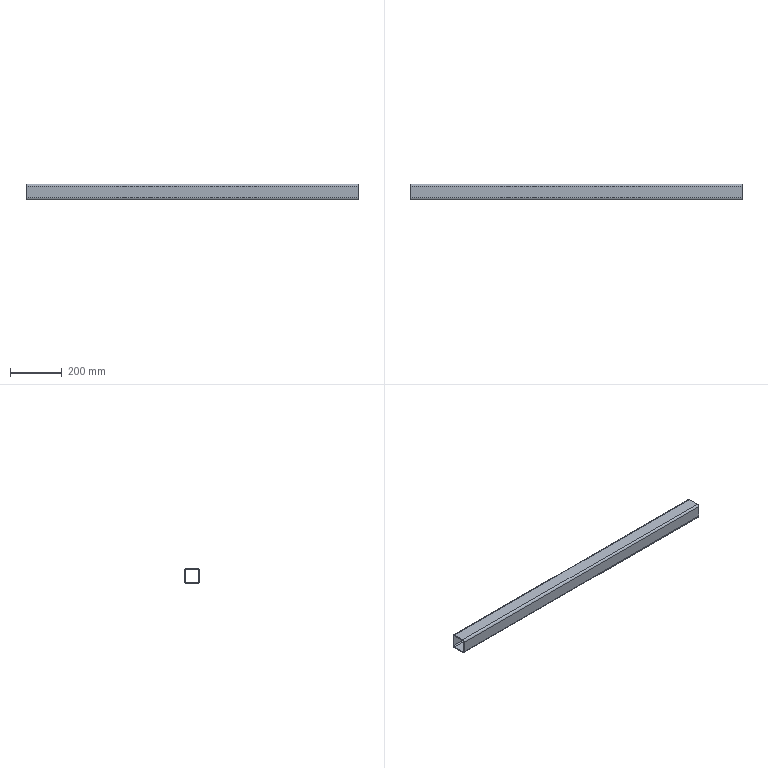Part | SolidWorks | features BaseBody 1 | 1 solid | 18 faces | box 1280 x 60 x 60 mm | volume 1094139 mm3 | plane 10 | cylinder 8 | commonest cylinder face diameters 8 x4 16 x4
STEP:
#1=CARTESIAN_POINT('',(640.,44.,-4.));
#2=VERTEX_POINT('',#1);
#3=CARTESIAN_POINT('',(640.,0.,-4.));
#4=VERTEX_POINT('',#3);
#5=CARTESIAN_POINT('',(640.,44.,-4.));
#6=DIRECTION('',(0.,-1.,0.));
#7=VECTOR('',#6,1000.);
#8=LINE('',#5,#7);
#9=EDGE_CURVE('',#2,#4,#8,.T.);
#10=ORIENTED_EDGE('',*,*,#9,.T.);
#11=CARTESIAN_POINT('',(-640.,0.,-4.));
#12=VERTEX_POINT('',#11);
#13=CARTESIAN_POINT('',(670.,0.,-4.));
#14=DIRECTION('',(-1.,0.,0.));
#15=VECTOR('',#14,1000.);
#16=LINE('',#13,#15);
#17=EDGE_CURVE('',#4,#12,#16,.T.);
#18=ORIENTED_EDGE('',*,*,#17,.T.);
#19=CARTESIAN_POINT('',(-640.,44.,-4.));
#20=VERTEX_POINT('',#19);
#21=CARTESIAN_POINT('',(-640.,44.,-4.));
#22=DIRECTION('',(0.,1.,0.));
#23=VECTOR('',#22,1000.);
#24=LINE('',#21,#23);
#25=EDGE_CURVE('',#12,#20,#24,.T.);
#26=ORIENTED_EDGE('',*,*,#25,.T.);
#27=CARTESIAN_POINT('',(670.,44.,-4.));
#28=DIRECTION('',(1.,0.,0.));
#29=VECTOR('',#28,1000.);
#30=LINE('',#27,#29);
#31=EDGE_CURVE('',#20,#2,#30,.T.);
#32=ORIENTED_EDGE('',*,*,#31,.T.);
#33=EDGE_LOOP('',(#10,#18,#26,#32));
#34=FACE_OUTER_BOUND('',#33,.T.);
#35=CARTESIAN_POINT('',(670.,44.,-4.));
#36=DIRECTION('',(0.,0.,-1.));
#37=DIRECTION('',(-1.,0.,0.));
#38=AXIS2_PLACEMENT_3D('',#35,#36,#37);
#39=PLANE('',#38);
#40=ADVANCED_FACE('',(#34),#39,.T.);
#41=ORIENTED_EDGE('',*,*,#17,.F.);
#42=CARTESIAN_POINT('',(640.,-4.,-8.));
#43=VERTEX_POINT('',#42);
#44=CARTESIAN_POINT('',(640.,0.,-8.));
#45=DIRECTION('',(-1.,0.,0.));
#46=DIRECTION('',(0.,0.,1.));
#47=AXIS2_PLACEMENT_3D('',#44,#45,#46);
#48=CIRCLE('',#47,4.);
#49=EDGE_CURVE('',#43,#4,#48,.T.);
#50=ORIENTED_EDGE('',*,*,#49,.F.);
#51=CARTESIAN_POINT('',(-640.,-4.,-8.));
#52=VERTEX_POINT('',#51);
#53=CARTESIAN_POINT('',(670.,-4.,-8.));
#54=DIRECTION('',(1.,0.,0.));
#55=VECTOR('',#54,1000.);
#56=LINE('',#53,#55);
#57=EDGE_CURVE('',#52,#43,#56,.T.);
#58=ORIENTED_EDGE('',*,*,#57,.F.);
#59=CARTESIAN_POINT('',(-640.,0.,-8.));
#60=DIRECTION('',(1.,0.,0.));
#61=DIRECTION('',(0.,0.,1.));
#62=AXIS2_PLACEMENT_3D('',#59,#60,#61);
#63=CIRCLE('',#62,4.);
#64=EDGE_CURVE('',#12,#52,#63,.T.);
#65=ORIENTED_EDGE('',*,*,#64,.F.);
#66=EDGE_LOOP('',(#41,#50,#58,#65));
#67=FACE_OUTER_BOUND('',#66,.T.);
#68=CARTESIAN_POINT('',(670.,0.,-8.));
#69=DIRECTION('',(-1.,0.,0.));
#70=DIRECTION('',(0.,0.,1.));
#71=AXIS2_PLACEMENT_3D('',#68,#69,#70);
#72=CYLINDRICAL_SURFACE('',#71,4.);
#73=ADVANCED_FACE('',(#67),#72,.F.);
#74=ORIENTED_EDGE('',*,*,#49,.T.);
#75=ORIENTED_EDGE('',*,*,#9,.F.);
#76=CARTESIAN_POINT('',(640.,48.,-8.));
#77=VERTEX_POINT('',#76);
#78=CARTESIAN_POINT('',(640.,44.,-8.));
#79=DIRECTION('',(-1.,0.,0.));
#80=DIRECTION('',(0.,0.,1.));
#81=AXIS2_PLACEMENT_3D('',#78,#79,#80);
#82=CIRCLE('',#81,4.);
#83=EDGE_CURVE('',#2,#77,#82,.T.);
#84=ORIENTED_EDGE('',*,*,#83,.T.);
#85=CARTESIAN_POINT('',(640.,48.,-52.));
#86=VERTEX_POINT('',#85);
#87=CARTESIAN_POINT('',(640.,48.,530.));
#88=DIRECTION('',(0.,0.,-1.));
#89=VECTOR('',#88,1000.);
#90=LINE('',#87,#89);
#91=EDGE_CURVE('',#77,#86,#90,.T.);
#92=ORIENTED_EDGE('',*,*,#91,.T.);
#93=CARTESIAN_POINT('',(640.,44.,-56.));
#94=VERTEX_POINT('',#93);
#95=CARTESIAN_POINT('',(640.,44.,-52.));
#96=DIRECTION('',(-1.,0.,0.));
#97=DIRECTION('',(0.,0.,1.));
#98=AXIS2_PLACEMENT_3D('',#95,#96,#97);
#99=CIRCLE('',#98,4.);
#100=EDGE_CURVE('',#86,#94,#99,.T.);
#101=ORIENTED_EDGE('',*,*,#100,.T.);
#102=CARTESIAN_POINT('',(640.,0.,-56.));
#103=VERTEX_POINT('',#102);
#104=CARTESIAN_POINT('',(640.,44.,-56.));
#105=DIRECTION('',(0.,-1.,0.));
#106=VECTOR('',#105,1000.);
#107=LINE('',#104,#106);
#108=EDGE_CURVE('',#94,#103,#107,.T.);
#109=ORIENTED_EDGE('',*,*,#108,.T.);
#110=CARTESIAN_POINT('',(640.,-4.,-52.));
#111=VERTEX_POINT('',#110);
#112=CARTESIAN_POINT('',(640.,0.,-52.));
#113=DIRECTION('',(-1.,0.,0.));
#114=DIRECTION('',(0.,0.,1.));
#115=AXIS2_PLACEMENT_3D('',#112,#113,#114);
#116=CIRCLE('',#115,4.);
#117=EDGE_CURVE('',#103,#111,#116,.T.);
#118=ORIENTED_EDGE('',*,*,#117,.T.);
#119=CARTESIAN_POINT('',(640.,-4.,530.));
#120=DIRECTION('',(0.,0.,1.));
#121=VECTOR('',#120,1000.);
#122=LINE('',#119,#121);
#123=EDGE_CURVE('',#111,#43,#122,.T.);
#124=ORIENTED_EDGE('',*,*,#123,.T.);
#125=EDGE_LOOP('',(#74,#75,#84,#92,#101,#109,#118,#124));
#126=FACE_BOUND('',#125,.T.);
#127=CARTESIAN_POINT('',(640.,52.,-52.));
#128=VERTEX_POINT('',#127);
#129=CARTESIAN_POINT('',(640.,52.,-8.));
#130=VERTEX_POINT('',#129);
#131=CARTESIAN_POINT('',(640.,52.,530.));
#132=DIRECTION('',(0.,0.,1.));
#133=VECTOR('',#132,1000.);
#134=LINE('',#131,#133);
#135=EDGE_CURVE('',#128,#130,#134,.T.);
#136=ORIENTED_EDGE('',*,*,#135,.T.);
#137=CARTESIAN_POINT('',(640.,44.,0.));
#138=VERTEX_POINT('',#137);
#139=CARTESIAN_POINT('',(640.,44.,-8.));
#140=DIRECTION('',(1.,0.,0.));
#141=DIRECTION('',(0.,0.,1.));
#142=AXIS2_PLACEMENT_3D('',#139,#140,#141);
#143=CIRCLE('',#142,8.);
#144=EDGE_CURVE('',#130,#138,#143,.T.);
#145=ORIENTED_EDGE('',*,*,#144,.T.);
#146=CARTESIAN_POINT('',(640.,0.,0.));
#147=VERTEX_POINT('',#146);
#148=CARTESIAN_POINT('',(640.,44.,0.));
#149=DIRECTION('',(0.,-1.,0.));
#150=VECTOR('',#149,1000.);
#151=LINE('',#148,#150);
#152=EDGE_CURVE('',#138,#147,#151,.T.);
#153=ORIENTED_EDGE('',*,*,#152,.T.);
#154=CARTESIAN_POINT('',(640.,-8.,-8.));
#155=VERTEX_POINT('',#154);
#156=CARTESIAN_POINT('',(640.,0.,-8.));
#157=DIRECTION('',(1.,0.,0.));
#158=DIRECTION('',(0.,0.,1.));
#159=AXIS2_PLACEMENT_3D('',#156,#157,#158);
#160=CIRCLE('',#159,8.);
#161=EDGE_CURVE('',#147,#155,#160,.T.);
#162=ORIENTED_EDGE('',*,*,#161,.T.);
#163=CARTESIAN_POINT('',(640.,-8.,-52.));
#164=VERTEX_POINT('',#163);
#165=CARTESIAN_POINT('',(640.,-8.,530.));
#166=DIRECTION('',(0.,0.,-1.));
#167=VECTOR('',#166,1000.);
#168=LINE('',#165,#167);
#169=EDGE_CURVE('',#155,#164,#168,.T.);
#170=ORIENTED_EDGE('',*,*,#169,.T.);
#171=CARTESIAN_POINT('',(640.,0.,-60.));
#172=VERTEX_POINT('',#171);
#173=CARTESIAN_POINT('',(640.,0.,-52.));
#174=DIRECTION('',(1.,0.,0.));
#175=DIRECTION('',(0.,0.,1.));
#176=AXIS2_PLACEMENT_3D('',#173,#174,#175);
#177=CIRCLE('',#176,8.);
#178=EDGE_CURVE('',#164,#172,#177,.T.);
#179=ORIENTED_EDGE('',*,*,#178,.T.);
#180=CARTESIAN_POINT('',(640.,44.,-60.));
#181=VERTEX_POINT('',#180);
#182=CARTESIAN_POINT('',(640.,44.,-60.));
#183=DIRECTION('',(0.,1.,0.));
#184=VECTOR('',#183,1000.);
#185=LINE('',#182,#184);
#186=EDGE_CURVE('',#172,#181,#185,.T.);
#187=ORIENTED_EDGE('',*,*,#186,.T.);
#188=CARTESIAN_POINT('',(640.,44.,-52.));
#189=DIRECTION('',(1.,0.,0.));
#190=DIRECTION('',(0.,0.,1.));
#191=AXIS2_PLACEMENT_3D('',#188,#189,#190);
#192=CIRCLE('',#191,8.);
#193=EDGE_CURVE('',#181,#128,#192,.T.);
#194=ORIENTED_EDGE('',*,*,#193,.T.);
#195=EDGE_LOOP('',(#136,#145,#153,#162,#170,#179,#187,#194));
#196=FACE_OUTER_BOUND('',#195,.T.);
#197=CARTESIAN_POINT('',(640.,44.,530.));
#198=DIRECTION('',(1.,0.,0.));
#199=DIRECTION('',(0.,0.,-1.));
#200=AXIS2_PLACEMENT_3D('',#197,#198,#199);
#201=PLANE('',#200);
#202=ADVANCED_FACE('',(#126,#196),#201,.T.);
#203=CARTESIAN_POINT('',(-640.,48.,-8.));
#204=VERTEX_POINT('',#203);
#205=CARTESIAN_POINT('',(670.,48.,-8.));
#206=DIRECTION('',(-1.,0.,0.));
#207=VECTOR('',#206,1000.);
#208=LINE('',#205,#207);
#209=EDGE_CURVE('',#77,#204,#208,.T.);
#210=ORIENTED_EDGE('',*,*,#209,.F.);
#211=ORIENTED_EDGE('',*,*,#83,.F.);
#212=ORIENTED_EDGE('',*,*,#31,.F.);
#213=CARTESIAN_POINT('',(-640.,44.,-8.));
#214=DIRECTION('',(1.,0.,0.));
#215=DIRECTION('',(0.,0.,1.));
#216=AXIS2_PLACEMENT_3D('',#213,#214,#215);
#217=CIRCLE('',#216,4.);
#218=EDGE_CURVE('',#204,#20,#217,.T.);
#219=ORIENTED_EDGE('',*,*,#218,.F.);
#220=EDGE_LOOP('',(#210,#211,#212,#219));
#221=FACE_OUTER_BOUND('',#220,.T.);
#222=CARTESIAN_POINT('',(670.,44.,-8.));
#223=DIRECTION('',(-1.,0.,0.));
#224=DIRECTION('',(0.,0.,1.));
#225=AXIS2_PLACEMENT_3D('',#222,#223,#224);
#226=CYLINDRICAL_SURFACE('',#225,4.);
#227=ADVANCED_FACE('',(#221),#226,.F.);
#228=CARTESIAN_POINT('',(-640.,-4.,-52.));
#229=VERTEX_POINT('',#228);
#230=CARTESIAN_POINT('',(-640.,-4.,530.));
#231=DIRECTION('',(0.,0.,-1.));
#232=VECTOR('',#231,1000.);
#233=LINE('',#230,#232);
#234=EDGE_CURVE('',#52,#229,#233,.T.);
#235=ORIENTED_EDGE('',*,*,#234,.T.);
#236=CARTESIAN_POINT('',(-640.,0.,-56.));
#237=VERTEX_POINT('',#236);
#238=CARTESIAN_POINT('',(-640.,0.,-52.));
#239=DIRECTION('',(1.,0.,0.));
#240=DIRECTION('',(0.,0.,1.));
#241=AXIS2_PLACEMENT_3D('',#238,#239,#240);
#242=CIRCLE('',#241,4.);
#243=EDGE_CURVE('',#229,#237,#242,.T.);
#244=ORIENTED_EDGE('',*,*,#243,.T.);
#245=CARTESIAN_POINT('',(-640.,44.,-56.));
#246=VERTEX_POINT('',#245);
#247=CARTESIAN_POINT('',(-640.,0.,-56.));
#248=DIRECTION('',(0.,1.,0.));
#249=VECTOR('',#248,1000.);
#250=LINE('',#247,#249);
#251=EDGE_CURVE('',#237,#246,#250,.T.);
#252=ORIENTED_EDGE('',*,*,#251,.T.);
#253=CARTESIAN_POINT('',(-640.,48.,-52.));
#254=VERTEX_POINT('',#253);
#255=CARTESIAN_POINT('',(-640.,44.,-52.));
#256=DIRECTION('',(1.,0.,0.));
#257=DIRECTION('',(0.,0.,1.));
#258=AXIS2_PLACEMENT_3D('',#255,#256,#257);
#259=CIRCLE('',#258,4.);
#260=EDGE_CURVE('',#246,#254,#259,.T.);
#261=ORIENTED_EDGE('',*,*,#260,.T.);
#262=CARTESIAN_POINT('',(-640.,48.,530.));
#263=DIRECTION('',(0.,0.,1.));
#264=VECTOR('',#263,1000.);
#265=LINE('',#262,#264);
#266=EDGE_CURVE('',#254,#204,#265,.T.);
#267=ORIENTED_EDGE('',*,*,#266,.T.);
#268=ORIENTED_EDGE('',*,*,#218,.T.);
#269=ORIENTED_EDGE('',*,*,#25,.F.);
#270=ORIENTED_EDGE('',*,*,#64,.T.);
#271=EDGE_LOOP('',(#235,#244,#252,#261,#267,#268,#269,#270));
#272=FACE_BOUND('',#271,.T.);
#273=CARTESIAN_POINT('',(-640.,52.,-8.));
#274=VERTEX_POINT('',#273);
#275=CARTESIAN_POINT('',(-640.,52.,-52.));
#276=VERTEX_POINT('',#275);
#277=CARTESIAN_POINT('',(-640.,52.,530.));
#278=DIRECTION('',(0.,0.,-1.));
#279=VECTOR('',#278,1000.);
#280=LINE('',#277,#279);
#281=EDGE_CURVE('',#274,#276,#280,.T.);
#282=ORIENTED_EDGE('',*,*,#281,.T.);
#283=CARTESIAN_POINT('',(-640.,44.,-60.));
#284=VERTEX_POINT('',#283);
#285=CARTESIAN_POINT('',(-640.,44.,-52.));
#286=DIRECTION('',(-1.,0.,0.));
#287=DIRECTION('',(0.,0.,1.));
#288=AXIS2_PLACEMENT_3D('',#285,#286,#287);
#289=CIRCLE('',#288,8.);
#290=EDGE_CURVE('',#276,#284,#289,.T.);
#291=ORIENTED_EDGE('',*,*,#290,.T.);
#292=CARTESIAN_POINT('',(-640.,0.,-60.));
#293=VERTEX_POINT('',#292);
#294=CARTESIAN_POINT('',(-640.,0.,-60.));
#295=DIRECTION('',(0.,-1.,0.));
#296=VECTOR('',#295,1000.);
#297=LINE('',#294,#296);
#298=EDGE_CURVE('',#284,#293,#297,.T.);
#299=ORIENTED_EDGE('',*,*,#298,.T.);
#300=CARTESIAN_POINT('',(-640.,-8.,-52.));
#301=VERTEX_POINT('',#300);
#302=CARTESIAN_POINT('',(-640.,0.,-52.));
#303=DIRECTION('',(-1.,0.,0.));
#304=DIRECTION('',(0.,0.,1.));
#305=AXIS2_PLACEMENT_3D('',#302,#303,#304);
#306=CIRCLE('',#305,8.);
#307=EDGE_CURVE('',#293,#301,#306,.T.);
#308=ORIENTED_EDGE('',*,*,#307,.T.);
#309=CARTESIAN_POINT('',(-640.,-8.,-8.));
#310=VERTEX_POINT('',#309);
#311=CARTESIAN_POINT('',(-640.,-8.,530.));
#312=DIRECTION('',(0.,0.,1.));
#313=VECTOR('',#312,1000.);
#314=LINE('',#311,#313);
#315=EDGE_CURVE('',#301,#310,#314,.T.);
#316=ORIENTED_EDGE('',*,*,#315,.T.);
#317=CARTESIAN_POINT('',(-640.,0.,0.));
#318=VERTEX_POINT('',#317);
#319=CARTESIAN_POINT('',(-640.,0.,-8.));
#320=DIRECTION('',(-1.,0.,0.));
#321=DIRECTION('',(0.,0.,1.));
#322=AXIS2_PLACEMENT_3D('',#319,#320,#321);
#323=CIRCLE('',#322,8.);
#324=EDGE_CURVE('',#310,#318,#323,.T.);
#325=ORIENTED_EDGE('',*,*,#324,.T.);
#326=CARTESIAN_POINT('',(-640.,44.,0.));
#327=VERTEX_POINT('',#326);
#328=CARTESIAN_POINT('',(-640.,0.,0.));
#329=DIRECTION('',(0.,1.,0.));
#330=VECTOR('',#329,1000.);
#331=LINE('',#328,#330);
#332=EDGE_CURVE('',#318,#327,#331,.T.);
#333=ORIENTED_EDGE('',*,*,#332,.T.);
#334=CARTESIAN_POINT('',(-640.,44.,-8.));
#335=DIRECTION('',(-1.,0.,0.));
#336=DIRECTION('',(0.,0.,1.));
#337=AXIS2_PLACEMENT_3D('',#334,#335,#336);
#338=CIRCLE('',#337,8.);
#339=EDGE_CURVE('',#327,#274,#338,.T.);
#340=ORIENTED_EDGE('',*,*,#339,.T.);
#341=EDGE_LOOP('',(#282,#291,#299,#308,#316,#325,#333,#340));
#342=FACE_OUTER_BOUND('',#341,.T.);
#343=CARTESIAN_POINT('',(-640.,0.,530.));
#344=DIRECTION('',(-1.,0.,0.));
#345=DIRECTION('',(0.,0.,1.));
#346=AXIS2_PLACEMENT_3D('',#343,#344,#345);
#347=PLANE('',#346);
#348=ADVANCED_FACE('',(#272,#342),#347,.T.);
#349=ORIENTED_EDGE('',*,*,#123,.F.);
#350=CARTESIAN_POINT('',(670.,-4.,-52.));
#351=DIRECTION('',(-1.,0.,0.));
#352=VECTOR('',#351,1000.);
#353=LINE('',#350,#352);
#354=EDGE_CURVE('',#111,#229,#353,.T.);
#355=ORIENTED_EDGE('',*,*,#354,.T.);
#356=ORIENTED_EDGE('',*,*,#234,.F.);
#357=ORIENTED_EDGE('',*,*,#57,.T.);
#358=EDGE_LOOP('',(#349,#355,#356,#357));
#359=FACE_OUTER_BOUND('',#358,.T.);
#360=CARTESIAN_POINT('',(670.,-4.,-52.));
#361=DIRECTION('',(0.,1.,0.));
#362=DIRECTION('',(0.,0.,1.));
#363=AXIS2_PLACEMENT_3D('',#360,#361,#362);
#364=PLANE('',#363);
#365=ADVANCED_FACE('',(#359),#364,.T.);
#366=ORIENTED_EDGE('',*,*,#354,.F.);
#367=ORIENTED_EDGE('',*,*,#117,.F.);
#368=CARTESIAN_POINT('',(670.,0.,-56.));
#369=DIRECTION('',(1.,0.,0.));
#370=VECTOR('',#369,1000.);
#371=LINE('',#368,#370);
#372=EDGE_CURVE('',#237,#103,#371,.T.);
#373=ORIENTED_EDGE('',*,*,#372,.F.);
#374=ORIENTED_EDGE('',*,*,#243,.F.);
#375=EDGE_LOOP('',(#366,#367,#373,#374));
#376=FACE_OUTER_BOUND('',#375,.T.);
#377=CARTESIAN_POINT('',(670.,0.,-52.));
#378=DIRECTION('',(-1.,0.,0.));
#379=DIRECTION('',(0.,0.,1.));
#380=AXIS2_PLACEMENT_3D('',#377,#378,#379);
#381=CYLINDRICAL_SURFACE('',#380,4.);
#382=ADVANCED_FACE('',(#376),#381,.F.);
#383=ORIENTED_EDGE('',*,*,#108,.F.);
#384=CARTESIAN_POINT('',(670.,44.,-56.));
#385=DIRECTION('',(-1.,0.,0.));
#386=VECTOR('',#385,1000.);
#387=LINE('',#384,#386);
#388=EDGE_CURVE('',#94,#246,#387,.T.);
#389=ORIENTED_EDGE('',*,*,#388,.T.);
#390=ORIENTED_EDGE('',*,*,#251,.F.);
#391=ORIENTED_EDGE('',*,*,#372,.T.);
#392=EDGE_LOOP('',(#383,#389,#390,#391));
#393=FACE_OUTER_BOUND('',#392,.T.);
#394=CARTESIAN_POINT('',(670.,0.,-56.));
#395=DIRECTION('',(0.,0.,1.));
#396=DIRECTION('',(1.,0.,0.));
#397=AXIS2_PLACEMENT_3D('',#394,#395,#396);
#398=PLANE('',#397);
#399=ADVANCED_FACE('',(#393),#398,.T.);
#400=ORIENTED_EDGE('',*,*,#388,.F.);
#401=ORIENTED_EDGE('',*,*,#100,.F.);
#402=CARTESIAN_POINT('',(670.,48.,-52.));
#403=DIRECTION('',(1.,0.,0.));
#404=VECTOR('',#403,1000.);
#405=LINE('',#402,#404);
#406=EDGE_CURVE('',#254,#86,#405,.T.);
#407=ORIENTED_EDGE('',*,*,#406,.F.);
#408=ORIENTED_EDGE('',*,*,#260,.F.);
#409=EDGE_LOOP('',(#400,#401,#407,#408));
#410=FACE_OUTER_BOUND('',#409,.T.);
#411=CARTESIAN_POINT('',(670.,44.,-52.));
#412=DIRECTION('',(-1.,0.,0.));
#413=DIRECTION('',(0.,0.,1.));
#414=AXIS2_PLACEMENT_3D('',#411,#412,#413);
#415=CYLINDRICAL_SURFACE('',#414,4.);
#416=ADVANCED_FACE('',(#410),#415,.F.);
#417=ORIENTED_EDGE('',*,*,#91,.F.);
#418=ORIENTED_EDGE('',*,*,#209,.T.);
#419=ORIENTED_EDGE('',*,*,#266,.F.);
#420=ORIENTED_EDGE('',*,*,#406,.T.);
#421=EDGE_LOOP('',(#417,#418,#419,#420));
#422=FACE_OUTER_BOUND('',#421,.T.);
#423=CARTESIAN_POINT('',(670.,48.,-8.));
#424=DIRECTION('',(0.,-1.,0.));
#425=DIRECTION('',(0.,0.,-1.));
#426=AXIS2_PLACEMENT_3D('',#423,#424,#425);
#427=PLANE('',#426);
#428=ADVANCED_FACE('',(#422),#427,.T.);
#429=CARTESIAN_POINT('',(670.,52.,-8.));
#430=DIRECTION('',(-1.,0.,0.));
#431=VECTOR('',#430,1000.);
#432=LINE('',#429,#431);
#433=EDGE_CURVE('',#130,#274,#432,.T.);
#434=ORIENTED_EDGE('',*,*,#433,.T.);
#435=ORIENTED_EDGE('',*,*,#339,.F.);
#436=CARTESIAN_POINT('',(670.,44.,0.));
#437=DIRECTION('',(1.,0.,0.));
#438=VECTOR('',#437,1000.);
#439=LINE('',#436,#438);
#440=EDGE_CURVE('',#327,#138,#439,.T.);
#441=ORIENTED_EDGE('',*,*,#440,.T.);
#442=ORIENTED_EDGE('',*,*,#144,.F.);
#443=EDGE_LOOP('',(#434,#435,#441,#442));
#444=FACE_OUTER_BOUND('',#443,.T.);
#445=CARTESIAN_POINT('',(670.,44.,-8.));
#446=DIRECTION('',(-1.,0.,0.));
#447=DIRECTION('',(0.,0.,1.));
#448=AXIS2_PLACEMENT_3D('',#445,#446,#447);
#449=CYLINDRICAL_SURFACE('',#448,8.);
#450=ADVANCED_FACE('',(#444),#449,.T.);
#451=ORIENTED_EDGE('',*,*,#135,.F.);
#452=CARTESIAN_POINT('',(670.,52.,-52.));
#453=DIRECTION('',(1.,0.,0.));
#454=VECTOR('',#453,1000.);
#455=LINE('',#452,#454);
#456=EDGE_CURVE('',#276,#128,#455,.T.);
#457=ORIENTED_EDGE('',*,*,#456,.F.);
#458=ORIENTED_EDGE('',*,*,#281,.F.);
#459=ORIENTED_EDGE('',*,*,#433,.F.);
#460=EDGE_LOOP('',(#451,#457,#458,#459));
#461=FACE_OUTER_BOUND('',#460,.T.);
#462=CARTESIAN_POINT('',(670.,52.,-8.));
#463=DIRECTION('',(0.,-1.,0.));
#464=DIRECTION('',(0.,0.,-1.));
#465=AXIS2_PLACEMENT_3D('',#462,#463,#464);
#466=PLANE('',#465);
#467=ADVANCED_FACE('',(#461),#466,.F.);
#468=CARTESIAN_POINT('',(670.,44.,-60.));
#469=DIRECTION('',(-1.,0.,0.));
#470=VECTOR('',#469,1000.);
#471=LINE('',#468,#470);
#472=EDGE_CURVE('',#181,#284,#471,.T.);
#473=ORIENTED_EDGE('',*,*,#472,.T.);
#474=ORIENTED_EDGE('',*,*,#290,.F.);
#475=ORIENTED_EDGE('',*,*,#456,.T.);
#476=ORIENTED_EDGE('',*,*,#193,.F.);
#477=EDGE_LOOP('',(#473,#474,#475,#476));
#478=FACE_OUTER_BOUND('',#477,.T.);
#479=CARTESIAN_POINT('',(670.,44.,-52.));
#480=DIRECTION('',(-1.,0.,0.));
#481=DIRECTION('',(0.,0.,1.));
#482=AXIS2_PLACEMENT_3D('',#479,#480,#481);
#483=CYLINDRICAL_SURFACE('',#482,8.);
#484=ADVANCED_FACE('',(#478),#483,.T.);
#485=ORIENTED_EDGE('',*,*,#186,.F.);
#486=CARTESIAN_POINT('',(670.,0.,-60.));
#487=DIRECTION('',(1.,0.,0.));
#488=VECTOR('',#487,1000.);
#489=LINE('',#486,#488);
#490=EDGE_CURVE('',#293,#172,#489,.T.);
#491=ORIENTED_EDGE('',*,*,#490,.F.);
#492=ORIENTED_EDGE('',*,*,#298,.F.);
#493=ORIENTED_EDGE('',*,*,#472,.F.);
#494=EDGE_LOOP('',(#485,#491,#492,#493));
#495=FACE_OUTER_BOUND('',#494,.T.);
#496=CARTESIAN_POINT('',(670.,0.,-60.));
#497=DIRECTION('',(0.,0.,1.));
#498=DIRECTION('',(1.,0.,0.));
#499=AXIS2_PLACEMENT_3D('',#496,#497,#498);
#500=PLANE('',#499);
#501=ADVANCED_FACE('',(#495),#500,.F.);
#502=CARTESIAN_POINT('',(670.,-8.,-52.));
#503=DIRECTION('',(-1.,0.,0.));
#504=VECTOR('',#503,1000.);
#505=LINE('',#502,#504);
#506=EDGE_CURVE('',#164,#301,#505,.T.);
#507=ORIENTED_EDGE('',*,*,#506,.T.);
#508=ORIENTED_EDGE('',*,*,#307,.F.);
#509=ORIENTED_EDGE('',*,*,#490,.T.);
#510=ORIENTED_EDGE('',*,*,#178,.F.);
#511=EDGE_LOOP('',(#507,#508,#509,#510));
#512=FACE_OUTER_BOUND('',#511,.T.);
#513=CARTESIAN_POINT('',(670.,0.,-52.));
#514=DIRECTION('',(-1.,0.,0.));
#515=DIRECTION('',(0.,0.,1.));
#516=AXIS2_PLACEMENT_3D('',#513,#514,#515);
#517=CYLINDRICAL_SURFACE('',#516,8.);
#518=ADVANCED_FACE('',(#512),#517,.T.);
#519=ORIENTED_EDGE('',*,*,#169,.F.);
#520=CARTESIAN_POINT('',(670.,-8.,-8.));
#521=DIRECTION('',(1.,0.,0.));
#522=VECTOR('',#521,1000.);
#523=LINE('',#520,#522);
#524=EDGE_CURVE('',#310,#155,#523,.T.);
#525=ORIENTED_EDGE('',*,*,#524,.F.);
#526=ORIENTED_EDGE('',*,*,#315,.F.);
#527=ORIENTED_EDGE('',*,*,#506,.F.);
#528=EDGE_LOOP('',(#519,#525,#526,#527));
#529=FACE_OUTER_BOUND('',#528,.T.);
#530=CARTESIAN_POINT('',(670.,-8.,-52.));
#531=DIRECTION('',(0.,1.,0.));
#532=DIRECTION('',(0.,0.,1.));
#533=AXIS2_PLACEMENT_3D('',#530,#531,#532);
#534=PLANE('',#533);
#535=ADVANCED_FACE('',(#529),#534,.F.);
#536=CARTESIAN_POINT('',(670.,0.,0.));
#537=DIRECTION('',(-1.,0.,0.));
#538=VECTOR('',#537,1000.);
#539=LINE('',#536,#538);
#540=EDGE_CURVE('',#147,#318,#539,.T.);
#541=ORIENTED_EDGE('',*,*,#540,.T.);
#542=ORIENTED_EDGE('',*,*,#324,.F.);
#543=ORIENTED_EDGE('',*,*,#524,.T.);
#544=ORIENTED_EDGE('',*,*,#161,.F.);
#545=EDGE_LOOP('',(#541,#542,#543,#544));
#546=FACE_OUTER_BOUND('',#545,.T.);
#547=CARTESIAN_POINT('',(670.,0.,-8.));
#548=DIRECTION('',(-1.,0.,0.));
#549=DIRECTION('',(0.,0.,1.));
#550=AXIS2_PLACEMENT_3D('',#547,#548,#549);
#551=CYLINDRICAL_SURFACE('',#550,8.);
#552=ADVANCED_FACE('',(#546),#551,.T.);
#553=ORIENTED_EDGE('',*,*,#152,.F.);
#554=ORIENTED_EDGE('',*,*,#440,.F.);
#555=ORIENTED_EDGE('',*,*,#332,.F.);
#556=ORIENTED_EDGE('',*,*,#540,.F.);
#557=EDGE_LOOP('',(#553,#554,#555,#556));
#558=FACE_OUTER_BOUND('',#557,.T.);
#559=CARTESIAN_POINT('',(670.,44.,0.));
#560=DIRECTION('',(0.,0.,-1.));
#561=DIRECTION('',(-1.,0.,0.));
#562=AXIS2_PLACEMENT_3D('',#559,#560,#561);
#563=PLANE('',#562);
#564=ADVANCED_FACE('',(#558),#563,.F.);
#565=CLOSED_SHELL('',(#40,#73,#202,#227,#348,#365,#382,#399,#416,#428,#450,#467,#484,#501,#518,#535,#552,#564));
#566=MANIFOLD_SOLID_BREP('',#565);
#567=CARTESIAN_POINT('',(0.,0.,0.));
#568=DIRECTION('',(0.,0.,1.));
#569=DIRECTION('',(1.,0.,0.));
#570=AXIS2_PLACEMENT_3D('',#567,#568,#569);
#571=(LENGTH_UNIT()NAMED_UNIT(*)SI_UNIT(.MILLI.,.METRE.));
#572=UNCERTAINTY_MEASURE_WITH_UNIT(LENGTH_MEASURE(0.00001),#571,'','');
#573=(NAMED_UNIT(*)PLANE_ANGLE_UNIT()SI_UNIT($,.RADIAN.));
#574=(NAMED_UNIT(*)SI_UNIT($,.STERADIAN.)SOLID_ANGLE_UNIT());
#575=(GEOMETRIC_REPRESENTATION_CONTEXT(3)GLOBAL_UNCERTAINTY_ASSIGNED_CONTEXT((#572))GLOBAL_UNIT_ASSIGNED_CONTEXT((#571,#573,#574))REPRESENTATION_CONTEXT('',''));
#576=ADVANCED_BREP_SHAPE_REPRESENTATION('',(#566,#570),#575);